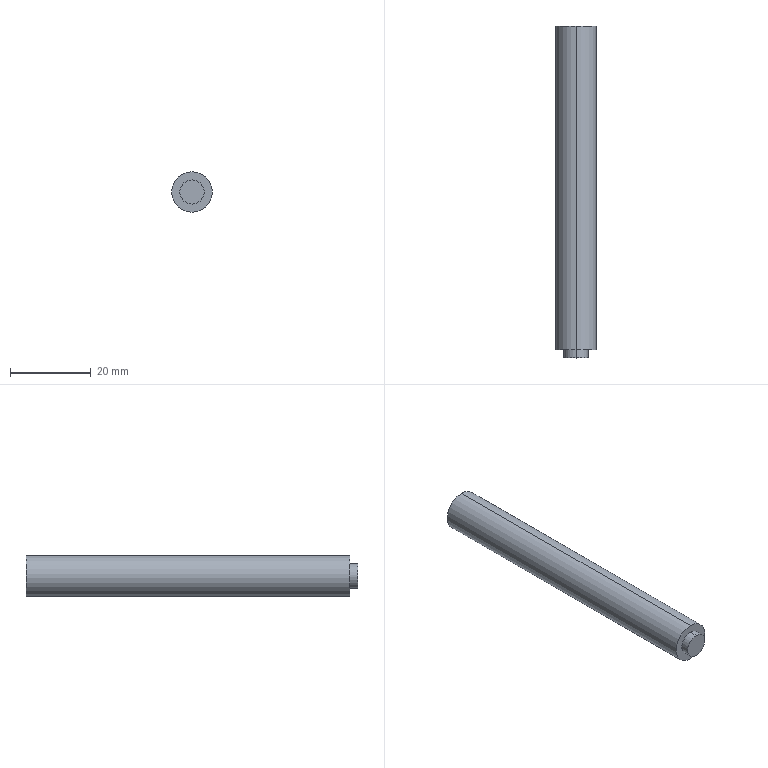Part | STEP file | 1 solid | 7 faces | box 10 x 82 x 10 mm | volume 6340 mm3 | cylinder 4 | plane 3 | commonest cylinder face diameters 6 x2 10 x2
STEP:
#1=CARTESIAN_POINT('',(0.,0.,0.));
#2=DIRECTION('',(0.,0.,1.));
#3=DIRECTION('',(1.,0.,0.));
#4=AXIS2_PLACEMENT_3D('',#1,#2,#3);
#5=CARTESIAN_POINT('',(0.,2.,5.));
#6=VERTEX_POINT('',#5);
#7=CARTESIAN_POINT('',(0.,2.,-5.));
#8=VERTEX_POINT('',#7);
#9=CARTESIAN_POINT('',(0.,2.,0.));
#10=DIRECTION('',(0.,1.,0.));
#11=DIRECTION('',(0.,0.,1.));
#12=AXIS2_PLACEMENT_3D('',#9,#10,#11);
#13=CIRCLE('',#12,5.);
#14=CARTESIAN_POINT('',(0.,2.,0.));
#15=DIRECTION('',(0.,1.,0.));
#16=DIRECTION('',(0.,0.,1.));
#17=AXIS2_PLACEMENT_3D('',#14,#15,#16);
#18=CYLINDRICAL_SURFACE('',#17,5.);
#19=CARTESIAN_POINT('',(0.,0.));
#20=DIRECTION('',(1.,0.));
#21=VECTOR('',#20,1.);
#22=LINE('',#19,#21);
#23=(GEOMETRIC_REPRESENTATION_CONTEXT(2)PARAMETRIC_REPRESENTATION_CONTEXT()REPRESENTATION_CONTEXT('',''));
#24=DEFINITIONAL_REPRESENTATION('',(#22),#23);
#25=PCURVE('',#18,#24);
#26=CARTESIAN_POINT('',(0.,2.,0.));
#27=DIRECTION('',(0.,1.,0.));
#28=DIRECTION('',(0.,0.,1.));
#29=AXIS2_PLACEMENT_3D('',#26,#27,#28);
#30=PLANE('',#29);
#31=CARTESIAN_POINT('',(0.,0.));
#32=DIRECTION('',(1.,0.));
#33=AXIS2_PLACEMENT_2D('',#31,#32);
#34=CIRCLE('',#33,5.);
#35=(GEOMETRIC_REPRESENTATION_CONTEXT(2)PARAMETRIC_REPRESENTATION_CONTEXT()REPRESENTATION_CONTEXT('',''));
#36=DEFINITIONAL_REPRESENTATION('',(#34),#35);
#37=PCURVE('',#30,#36);
#38=SURFACE_CURVE('',#13,(#25,#37),.PCURVE_S1.);
#39=EDGE_CURVE('',#6,#8,#38,.T.);
#40=ORIENTED_EDGE('',*,*,#39,.T.);
#41=CARTESIAN_POINT('',(0.,82.,-5.));
#42=VERTEX_POINT('',#41);
#43=CARTESIAN_POINT('',(0.,2.,-5.));
#44=DIRECTION('',(0.,1.,0.));
#45=VECTOR('',#44,1.);
#46=LINE('',#43,#45);
#47=CARTESIAN_POINT('',(3.142,0.));
#48=DIRECTION('',(0.,1.));
#49=VECTOR('',#48,1.);
#50=LINE('',#47,#49);
#51=(GEOMETRIC_REPRESENTATION_CONTEXT(2)PARAMETRIC_REPRESENTATION_CONTEXT()REPRESENTATION_CONTEXT('',''));
#52=DEFINITIONAL_REPRESENTATION('',(#50),#51);
#53=PCURVE('',#18,#52);
#54=CARTESIAN_POINT('',(0.,2.,0.));
#55=DIRECTION('',(0.,1.,0.));
#56=DIRECTION('',(0.,0.,1.));
#57=AXIS2_PLACEMENT_3D('',#54,#55,#56);
#58=CYLINDRICAL_SURFACE('',#57,5.);
#59=CARTESIAN_POINT('',(3.142,0.));
#60=DIRECTION('',(0.,1.));
#61=VECTOR('',#60,1.);
#62=LINE('',#59,#61);
#63=(GEOMETRIC_REPRESENTATION_CONTEXT(2)PARAMETRIC_REPRESENTATION_CONTEXT()REPRESENTATION_CONTEXT('',''));
#64=DEFINITIONAL_REPRESENTATION('',(#62),#63);
#65=PCURVE('',#58,#64);
#66=SURFACE_CURVE('',#46,(#53,#65),.PCURVE_S1.);
#67=EDGE_CURVE('',#8,#42,#66,.T.);
#68=ORIENTED_EDGE('',*,*,#67,.T.);
#69=CARTESIAN_POINT('',(0.,82.,5.));
#70=VERTEX_POINT('',#69);
#71=CARTESIAN_POINT('',(0.,82.,0.));
#72=DIRECTION('',(0.,-1.,0.));
#73=DIRECTION('',(0.,0.,1.));
#74=AXIS2_PLACEMENT_3D('',#71,#72,#73);
#75=CIRCLE('',#74,5.);
#76=CARTESIAN_POINT('',(6.283,80.));
#77=DIRECTION('',(-1.,0.));
#78=VECTOR('',#77,1.);
#79=LINE('',#76,#78);
#80=(GEOMETRIC_REPRESENTATION_CONTEXT(2)PARAMETRIC_REPRESENTATION_CONTEXT()REPRESENTATION_CONTEXT('',''));
#81=DEFINITIONAL_REPRESENTATION('',(#79),#80);
#82=PCURVE('',#18,#81);
#83=CARTESIAN_POINT('',(0.,82.,0.));
#84=DIRECTION('',(0.,1.,0.));
#85=DIRECTION('',(0.,0.,1.));
#86=AXIS2_PLACEMENT_3D('',#83,#84,#85);
#87=PLANE('',#86);
#88=CARTESIAN_POINT('',(5.,0.));
#89=CARTESIAN_POINT('',(5.,-8.66));
#90=CARTESIAN_POINT('',(-2.5,-4.33));
#91=CARTESIAN_POINT('',(-10.,0.));
#92=CARTESIAN_POINT('',(-2.5,4.33));
#93=CARTESIAN_POINT('',(5.,8.66));
#94=CARTESIAN_POINT('',(5.,0.));
#95=(BOUNDED_CURVE()B_SPLINE_CURVE(2,(#88,#89,#90,#91,#92,#93,#94),.UNSPECIFIED.,.T.,.F.)B_SPLINE_CURVE_WITH_KNOTS((1,2,2,2,2,1),(-2.094,0.,2.094,4.189,6.283,8.378),.UNSPECIFIED.)CURVE()GEOMETRIC_REPRESENTATION_ITEM()RATIONAL_B_SPLINE_CURVE((1.,0.5,1.,0.5,1.,0.5,1.))REPRESENTATION_ITEM(''));
#96=(GEOMETRIC_REPRESENTATION_CONTEXT(2)PARAMETRIC_REPRESENTATION_CONTEXT()REPRESENTATION_CONTEXT('',''));
#97=DEFINITIONAL_REPRESENTATION('',(#95),#96);
#98=PCURVE('',#87,#97);
#99=SURFACE_CURVE('',#75,(#82,#98),.PCURVE_S1.);
#100=EDGE_CURVE('',#42,#70,#99,.T.);
#101=ORIENTED_EDGE('',*,*,#100,.T.);
#102=CARTESIAN_POINT('',(0.,2.,5.));
#103=DIRECTION('',(0.,1.,0.));
#104=VECTOR('',#103,1.);
#105=LINE('',#102,#104);
#106=CARTESIAN_POINT('',(0.,0.));
#107=DIRECTION('',(0.,1.));
#108=VECTOR('',#107,1.);
#109=LINE('',#106,#108);
#110=(GEOMETRIC_REPRESENTATION_CONTEXT(2)PARAMETRIC_REPRESENTATION_CONTEXT()REPRESENTATION_CONTEXT('',''));
#111=DEFINITIONAL_REPRESENTATION('',(#109),#110);
#112=PCURVE('',#18,#111);
#113=CARTESIAN_POINT('',(6.283,0.));
#114=DIRECTION('',(0.,1.));
#115=VECTOR('',#114,1.);
#116=LINE('',#113,#115);
#117=(GEOMETRIC_REPRESENTATION_CONTEXT(2)PARAMETRIC_REPRESENTATION_CONTEXT()REPRESENTATION_CONTEXT('',''));
#118=DEFINITIONAL_REPRESENTATION('',(#116),#117);
#119=PCURVE('',#58,#118);
#120=SURFACE_CURVE('',#105,(#112,#119),.PCURVE_S1.);
#121=EDGE_CURVE('',#6,#70,#120,.T.);
#122=ORIENTED_EDGE('',*,*,#121,.F.);
#123=EDGE_LOOP('',(#40,#68,#101,#122));
#124=FACE_BOUND('',#123,.T.);
#125=ADVANCED_FACE('',(#124),#18,.T.);
#126=CARTESIAN_POINT('',(0.,0.,3.));
#127=VERTEX_POINT('',#126);
#128=CARTESIAN_POINT('',(0.,0.,-3.));
#129=VERTEX_POINT('',#128);
#130=CARTESIAN_POINT('',(0.,0.,0.));
#131=DIRECTION('',(0.,1.,0.));
#132=DIRECTION('',(0.,0.,1.));
#133=AXIS2_PLACEMENT_3D('',#130,#131,#132);
#134=CIRCLE('',#133,3.);
#135=CARTESIAN_POINT('',(0.,0.,0.));
#136=DIRECTION('',(0.,1.,0.));
#137=DIRECTION('',(0.,0.,1.));
#138=AXIS2_PLACEMENT_3D('',#135,#136,#137);
#139=CYLINDRICAL_SURFACE('',#138,3.);
#140=CARTESIAN_POINT('',(0.,0.));
#141=DIRECTION('',(1.,0.));
#142=VECTOR('',#141,1.);
#143=LINE('',#140,#142);
#144=(GEOMETRIC_REPRESENTATION_CONTEXT(2)PARAMETRIC_REPRESENTATION_CONTEXT()REPRESENTATION_CONTEXT('',''));
#145=DEFINITIONAL_REPRESENTATION('',(#143),#144);
#146=PCURVE('',#139,#145);
#147=CARTESIAN_POINT('',(0.,0.,0.));
#148=DIRECTION('',(0.,1.,0.));
#149=DIRECTION('',(0.,0.,1.));
#150=AXIS2_PLACEMENT_3D('',#147,#148,#149);
#151=PLANE('',#150);
#152=CARTESIAN_POINT('',(0.,0.));
#153=DIRECTION('',(1.,0.));
#154=AXIS2_PLACEMENT_2D('',#152,#153);
#155=CIRCLE('',#154,3.);
#156=(GEOMETRIC_REPRESENTATION_CONTEXT(2)PARAMETRIC_REPRESENTATION_CONTEXT()REPRESENTATION_CONTEXT('',''));
#157=DEFINITIONAL_REPRESENTATION('',(#155),#156);
#158=PCURVE('',#151,#157);
#159=SURFACE_CURVE('',#134,(#146,#158),.PCURVE_S1.);
#160=EDGE_CURVE('',#127,#129,#159,.T.);
#161=ORIENTED_EDGE('',*,*,#160,.T.);
#162=CARTESIAN_POINT('',(0.,2.,-3.));
#163=VERTEX_POINT('',#162);
#164=CARTESIAN_POINT('',(0.,0.,-3.));
#165=DIRECTION('',(0.,1.,0.));
#166=VECTOR('',#165,1.);
#167=LINE('',#164,#166);
#168=CARTESIAN_POINT('',(3.142,0.));
#169=DIRECTION('',(0.,1.));
#170=VECTOR('',#169,1.);
#171=LINE('',#168,#170);
#172=(GEOMETRIC_REPRESENTATION_CONTEXT(2)PARAMETRIC_REPRESENTATION_CONTEXT()REPRESENTATION_CONTEXT('',''));
#173=DEFINITIONAL_REPRESENTATION('',(#171),#172);
#174=PCURVE('',#139,#173);
#175=CARTESIAN_POINT('',(0.,0.,0.));
#176=DIRECTION('',(0.,1.,0.));
#177=DIRECTION('',(0.,0.,1.));
#178=AXIS2_PLACEMENT_3D('',#175,#176,#177);
#179=CYLINDRICAL_SURFACE('',#178,3.);
#180=CARTESIAN_POINT('',(3.142,0.));
#181=DIRECTION('',(0.,1.));
#182=VECTOR('',#181,1.);
#183=LINE('',#180,#182);
#184=(GEOMETRIC_REPRESENTATION_CONTEXT(2)PARAMETRIC_REPRESENTATION_CONTEXT()REPRESENTATION_CONTEXT('',''));
#185=DEFINITIONAL_REPRESENTATION('',(#183),#184);
#186=PCURVE('',#179,#185);
#187=SURFACE_CURVE('',#167,(#174,#186),.PCURVE_S1.);
#188=EDGE_CURVE('',#129,#163,#187,.T.);
#189=ORIENTED_EDGE('',*,*,#188,.T.);
#190=CARTESIAN_POINT('',(0.,2.,3.));
#191=VERTEX_POINT('',#190);
#192=CARTESIAN_POINT('',(0.,2.,0.));
#193=DIRECTION('',(0.,-1.,0.));
#194=DIRECTION('',(0.,0.,1.));
#195=AXIS2_PLACEMENT_3D('',#192,#193,#194);
#196=CIRCLE('',#195,3.);
#197=CARTESIAN_POINT('',(6.283,2.));
#198=DIRECTION('',(-1.,0.));
#199=VECTOR('',#198,1.);
#200=LINE('',#197,#199);
#201=(GEOMETRIC_REPRESENTATION_CONTEXT(2)PARAMETRIC_REPRESENTATION_CONTEXT()REPRESENTATION_CONTEXT('',''));
#202=DEFINITIONAL_REPRESENTATION('',(#200),#201);
#203=PCURVE('',#139,#202);
#204=CARTESIAN_POINT('',(3.,0.));
#205=CARTESIAN_POINT('',(3.,-5.196));
#206=CARTESIAN_POINT('',(-1.5,-2.598));
#207=CARTESIAN_POINT('',(-6.,0.));
#208=CARTESIAN_POINT('',(-1.5,2.598));
#209=CARTESIAN_POINT('',(3.,5.196));
#210=CARTESIAN_POINT('',(3.,0.));
#211=(BOUNDED_CURVE()B_SPLINE_CURVE(2,(#204,#205,#206,#207,#208,#209,#210),.UNSPECIFIED.,.T.,.F.)B_SPLINE_CURVE_WITH_KNOTS((1,2,2,2,2,1),(-2.094,0.,2.094,4.189,6.283,8.378),.UNSPECIFIED.)CURVE()GEOMETRIC_REPRESENTATION_ITEM()RATIONAL_B_SPLINE_CURVE((1.,0.5,1.,0.5,1.,0.5,1.))REPRESENTATION_ITEM(''));
#212=(GEOMETRIC_REPRESENTATION_CONTEXT(2)PARAMETRIC_REPRESENTATION_CONTEXT()REPRESENTATION_CONTEXT('',''));
#213=DEFINITIONAL_REPRESENTATION('',(#211),#212);
#214=PCURVE('',#30,#213);
#215=SURFACE_CURVE('',#196,(#203,#214),.PCURVE_S1.);
#216=EDGE_CURVE('',#163,#191,#215,.T.);
#217=ORIENTED_EDGE('',*,*,#216,.T.);
#218=CARTESIAN_POINT('',(0.,0.,3.));
#219=DIRECTION('',(0.,1.,0.));
#220=VECTOR('',#219,1.);
#221=LINE('',#218,#220);
#222=CARTESIAN_POINT('',(0.,0.));
#223=DIRECTION('',(0.,1.));
#224=VECTOR('',#223,1.);
#225=LINE('',#222,#224);
#226=(GEOMETRIC_REPRESENTATION_CONTEXT(2)PARAMETRIC_REPRESENTATION_CONTEXT()REPRESENTATION_CONTEXT('',''));
#227=DEFINITIONAL_REPRESENTATION('',(#225),#226);
#228=PCURVE('',#139,#227);
#229=CARTESIAN_POINT('',(6.283,0.));
#230=DIRECTION('',(0.,1.));
#231=VECTOR('',#230,1.);
#232=LINE('',#229,#231);
#233=(GEOMETRIC_REPRESENTATION_CONTEXT(2)PARAMETRIC_REPRESENTATION_CONTEXT()REPRESENTATION_CONTEXT('',''));
#234=DEFINITIONAL_REPRESENTATION('',(#232),#233);
#235=PCURVE('',#179,#234);
#236=SURFACE_CURVE('',#221,(#228,#235),.PCURVE_S1.);
#237=EDGE_CURVE('',#127,#191,#236,.T.);
#238=ORIENTED_EDGE('',*,*,#237,.F.);
#239=EDGE_LOOP('',(#161,#189,#217,#238));
#240=FACE_BOUND('',#239,.T.);
#241=ADVANCED_FACE('',(#240),#139,.T.);
#242=ORIENTED_EDGE('',*,*,#67,.F.);
#243=CARTESIAN_POINT('',(0.,2.,0.));
#244=DIRECTION('',(0.,1.,0.));
#245=DIRECTION('',(0.,0.,1.));
#246=AXIS2_PLACEMENT_3D('',#243,#244,#245);
#247=CIRCLE('',#246,5.);
#248=CARTESIAN_POINT('',(0.,0.));
#249=DIRECTION('',(1.,0.));
#250=VECTOR('',#249,1.);
#251=LINE('',#248,#250);
#252=(GEOMETRIC_REPRESENTATION_CONTEXT(2)PARAMETRIC_REPRESENTATION_CONTEXT()REPRESENTATION_CONTEXT('',''));
#253=DEFINITIONAL_REPRESENTATION('',(#251),#252);
#254=PCURVE('',#58,#253);
#255=CARTESIAN_POINT('',(0.,0.));
#256=DIRECTION('',(1.,0.));
#257=AXIS2_PLACEMENT_2D('',#255,#256);
#258=CIRCLE('',#257,5.);
#259=(GEOMETRIC_REPRESENTATION_CONTEXT(2)PARAMETRIC_REPRESENTATION_CONTEXT()REPRESENTATION_CONTEXT('',''));
#260=DEFINITIONAL_REPRESENTATION('',(#258),#259);
#261=PCURVE('',#30,#260);
#262=SURFACE_CURVE('',#247,(#254,#261),.PCURVE_S1.);
#263=EDGE_CURVE('',#8,#6,#262,.T.);
#264=ORIENTED_EDGE('',*,*,#263,.T.);
#265=ORIENTED_EDGE('',*,*,#121,.T.);
#266=CARTESIAN_POINT('',(0.,82.,0.));
#267=DIRECTION('',(0.,-1.,0.));
#268=DIRECTION('',(0.,0.,1.));
#269=AXIS2_PLACEMENT_3D('',#266,#267,#268);
#270=CIRCLE('',#269,5.);
#271=CARTESIAN_POINT('',(6.283,80.));
#272=DIRECTION('',(-1.,0.));
#273=VECTOR('',#272,1.);
#274=LINE('',#271,#273);
#275=(GEOMETRIC_REPRESENTATION_CONTEXT(2)PARAMETRIC_REPRESENTATION_CONTEXT()REPRESENTATION_CONTEXT('',''));
#276=DEFINITIONAL_REPRESENTATION('',(#274),#275);
#277=PCURVE('',#58,#276);
#278=CARTESIAN_POINT('',(5.,0.));
#279=CARTESIAN_POINT('',(5.,-8.66));
#280=CARTESIAN_POINT('',(-2.5,-4.33));
#281=CARTESIAN_POINT('',(-10.,0.));
#282=CARTESIAN_POINT('',(-2.5,4.33));
#283=CARTESIAN_POINT('',(5.,8.66));
#284=CARTESIAN_POINT('',(5.,0.));
#285=(BOUNDED_CURVE()B_SPLINE_CURVE(2,(#278,#279,#280,#281,#282,#283,#284),.UNSPECIFIED.,.T.,.F.)B_SPLINE_CURVE_WITH_KNOTS((1,2,2,2,2,1),(-2.094,0.,2.094,4.189,6.283,8.378),.UNSPECIFIED.)CURVE()GEOMETRIC_REPRESENTATION_ITEM()RATIONAL_B_SPLINE_CURVE((1.,0.5,1.,0.5,1.,0.5,1.))REPRESENTATION_ITEM(''));
#286=(GEOMETRIC_REPRESENTATION_CONTEXT(2)PARAMETRIC_REPRESENTATION_CONTEXT()REPRESENTATION_CONTEXT('',''));
#287=DEFINITIONAL_REPRESENTATION('',(#285),#286);
#288=PCURVE('',#87,#287);
#289=SURFACE_CURVE('',#270,(#277,#288),.PCURVE_S1.);
#290=EDGE_CURVE('',#70,#42,#289,.T.);
#291=ORIENTED_EDGE('',*,*,#290,.T.);
#292=EDGE_LOOP('',(#242,#264,#265,#291));
#293=FACE_BOUND('',#292,.T.);
#294=ADVANCED_FACE('',(#293),#58,.T.);
#295=CARTESIAN_POINT('',(0.,2.,0.));
#296=DIRECTION('',(0.,-1.,0.));
#297=DIRECTION('',(0.,0.,1.));
#298=AXIS2_PLACEMENT_3D('',#295,#296,#297);
#299=CIRCLE('',#298,3.);
#300=CARTESIAN_POINT('',(3.,0.));
#301=CARTESIAN_POINT('',(3.,-5.196));
#302=CARTESIAN_POINT('',(-1.5,-2.598));
#303=CARTESIAN_POINT('',(-6.,0.));
#304=CARTESIAN_POINT('',(-1.5,2.598));
#305=CARTESIAN_POINT('',(3.,5.196));
#306=CARTESIAN_POINT('',(3.,0.));
#307=(BOUNDED_CURVE()B_SPLINE_CURVE(2,(#300,#301,#302,#303,#304,#305,#306),.UNSPECIFIED.,.T.,.F.)B_SPLINE_CURVE_WITH_KNOTS((1,2,2,2,2,1),(-2.094,0.,2.094,4.189,6.283,8.378),.UNSPECIFIED.)CURVE()GEOMETRIC_REPRESENTATION_ITEM()RATIONAL_B_SPLINE_CURVE((1.,0.5,1.,0.5,1.,0.5,1.))REPRESENTATION_ITEM(''));
#308=(GEOMETRIC_REPRESENTATION_CONTEXT(2)PARAMETRIC_REPRESENTATION_CONTEXT()REPRESENTATION_CONTEXT('',''));
#309=DEFINITIONAL_REPRESENTATION('',(#307),#308);
#310=PCURVE('',#30,#309);
#311=CARTESIAN_POINT('',(6.283,2.));
#312=DIRECTION('',(-1.,0.));
#313=VECTOR('',#312,1.);
#314=LINE('',#311,#313);
#315=(GEOMETRIC_REPRESENTATION_CONTEXT(2)PARAMETRIC_REPRESENTATION_CONTEXT()REPRESENTATION_CONTEXT('',''));
#316=DEFINITIONAL_REPRESENTATION('',(#314),#315);
#317=PCURVE('',#179,#316);
#318=SURFACE_CURVE('',#299,(#310,#317),.PCURVE_S1.);
#319=EDGE_CURVE('',#191,#163,#318,.T.);
#320=ORIENTED_EDGE('',*,*,#319,.F.);
#321=ORIENTED_EDGE('',*,*,#216,.F.);
#322=EDGE_LOOP('',(#320,#321));
#323=FACE_BOUND('',#322,.T.);
#324=ORIENTED_EDGE('',*,*,#39,.F.);
#325=ORIENTED_EDGE('',*,*,#263,.F.);
#326=EDGE_LOOP('',(#324,#325));
#327=FACE_BOUND('',#326,.T.);
#328=ADVANCED_FACE('',(#323,#327),#30,.F.);
#329=ORIENTED_EDGE('',*,*,#290,.F.);
#330=ORIENTED_EDGE('',*,*,#100,.F.);
#331=EDGE_LOOP('',(#329,#330));
#332=FACE_BOUND('',#331,.T.);
#333=ADVANCED_FACE('',(#332),#87,.T.);
#334=ORIENTED_EDGE('',*,*,#188,.F.);
#335=CARTESIAN_POINT('',(0.,0.,0.));
#336=DIRECTION('',(0.,1.,0.));
#337=DIRECTION('',(0.,0.,1.));
#338=AXIS2_PLACEMENT_3D('',#335,#336,#337);
#339=CIRCLE('',#338,3.);
#340=CARTESIAN_POINT('',(0.,0.));
#341=DIRECTION('',(1.,0.));
#342=VECTOR('',#341,1.);
#343=LINE('',#340,#342);
#344=(GEOMETRIC_REPRESENTATION_CONTEXT(2)PARAMETRIC_REPRESENTATION_CONTEXT()REPRESENTATION_CONTEXT('',''));
#345=DEFINITIONAL_REPRESENTATION('',(#343),#344);
#346=PCURVE('',#179,#345);
#347=CARTESIAN_POINT('',(0.,0.));
#348=DIRECTION('',(1.,0.));
#349=AXIS2_PLACEMENT_2D('',#347,#348);
#350=CIRCLE('',#349,3.);
#351=(GEOMETRIC_REPRESENTATION_CONTEXT(2)PARAMETRIC_REPRESENTATION_CONTEXT()REPRESENTATION_CONTEXT('',''));
#352=DEFINITIONAL_REPRESENTATION('',(#350),#351);
#353=PCURVE('',#151,#352);
#354=SURFACE_CURVE('',#339,(#346,#353),.PCURVE_S1.);
#355=EDGE_CURVE('',#129,#127,#354,.T.);
#356=ORIENTED_EDGE('',*,*,#355,.T.);
#357=ORIENTED_EDGE('',*,*,#237,.T.);
#358=ORIENTED_EDGE('',*,*,#319,.T.);
#359=EDGE_LOOP('',(#334,#356,#357,#358));
#360=FACE_BOUND('',#359,.T.);
#361=ADVANCED_FACE('',(#360),#179,.T.);
#362=ORIENTED_EDGE('',*,*,#160,.F.);
#363=ORIENTED_EDGE('',*,*,#355,.F.);
#364=EDGE_LOOP('',(#362,#363));
#365=FACE_BOUND('',#364,.T.);
#366=ADVANCED_FACE('',(#365),#151,.F.);
#367=CLOSED_SHELL('',(#125,#241,#294,#328,#333,#361,#366));
#368=MANIFOLD_SOLID_BREP('',#367);
#369=(LENGTH_UNIT()NAMED_UNIT(*)SI_UNIT(.MILLI.,.METRE.));
#370=UNCERTAINTY_MEASURE_WITH_UNIT(LENGTH_MEASURE(0.0000001),#369,'','');
#371=(NAMED_UNIT(*)PLANE_ANGLE_UNIT()SI_UNIT($,.RADIAN.));
#372=(NAMED_UNIT(*)SI_UNIT($,.STERADIAN.)SOLID_ANGLE_UNIT());
#373=(GEOMETRIC_REPRESENTATION_CONTEXT(3)GLOBAL_UNCERTAINTY_ASSIGNED_CONTEXT((#370))GLOBAL_UNIT_ASSIGNED_CONTEXT((#369,#371,#372))REPRESENTATION_CONTEXT('',''));
#374=ADVANCED_BREP_SHAPE_REPRESENTATION('',(#4,#368),#373);